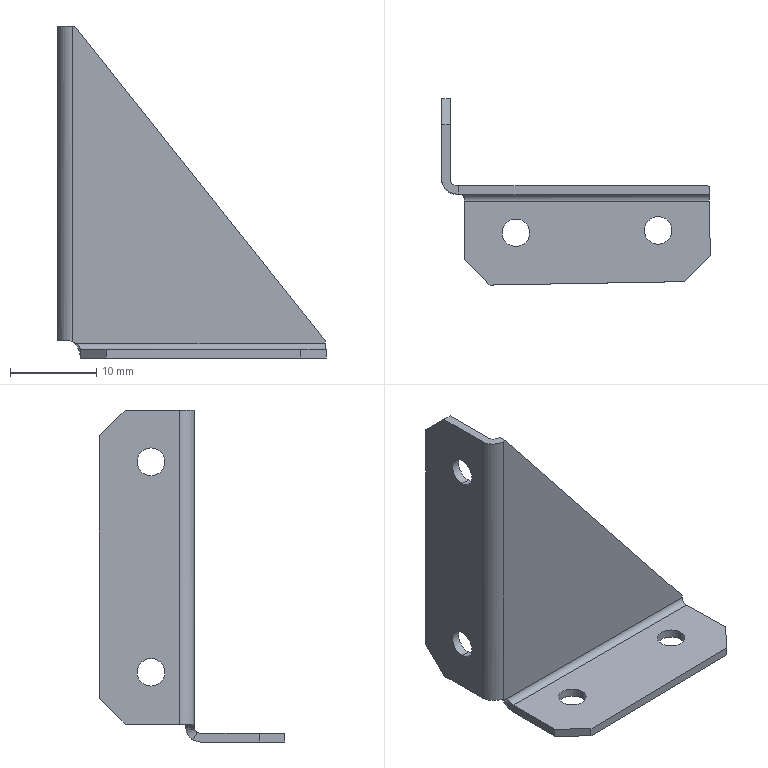Part | SolidWorks | features BaseBody 1 | 1 solid | 34 faces | box 31.131 x 21.506 x 38.476 mm | volume 1233 mm3 | plane 18 | cylinder 13 | spline 3 | commonest cylinder face diameters 3.2 x9 1.473 x2 3.473 x2
STEP:
#1=CARTESIAN_POINT('',(6.,-5.422,0.5237));
#2=VERTEX_POINT('',#1);
#3=CARTESIAN_POINT('',(9.2,-5.422,0.5237));
#4=VERTEX_POINT('',#3);
#5=CARTESIAN_POINT('',(7.6,-5.422,0.5237));
#6=DIRECTION('',(0.,0.,1.));
#7=DIRECTION('',(-1.,0.,0.));
#8=AXIS2_PLACEMENT_3D('',#5,#6,#7);
#9=CIRCLE('',#8,1.6);
#10=EDGE_CURVE('',#2,#4,#9,.T.);
#11=ORIENTED_EDGE('',*,*,#10,.T.);
#12=CARTESIAN_POINT('',(9.2,-5.422,-0.4763));
#13=VERTEX_POINT('',#12);
#14=CARTESIAN_POINT('',(9.2,-5.422,0.5237));
#15=DIRECTION('',(0.,0.,-1.));
#16=VECTOR('',#15,1000.);
#17=LINE('',#14,#16);
#18=EDGE_CURVE('',#4,#13,#17,.T.);
#19=ORIENTED_EDGE('',*,*,#18,.T.);
#20=CARTESIAN_POINT('',(6.,-5.422,-0.4763));
#21=VERTEX_POINT('',#20);
#22=CARTESIAN_POINT('',(7.6,-5.422,-0.4763));
#23=DIRECTION('',(0.,0.,-1.));
#24=DIRECTION('',(-1.,0.,0.));
#25=AXIS2_PLACEMENT_3D('',#22,#23,#24);
#26=CIRCLE('',#25,1.6);
#27=EDGE_CURVE('',#13,#21,#26,.T.);
#28=ORIENTED_EDGE('',*,*,#27,.T.);
#29=CARTESIAN_POINT('',(6.,-5.422,0.5237));
#30=DIRECTION('',(0.,0.,-1.));
#31=VECTOR('',#30,1000.);
#32=LINE('',#29,#31);
#33=EDGE_CURVE('',#2,#21,#32,.T.);
#34=ORIENTED_EDGE('',*,*,#33,.F.);
#35=EDGE_LOOP('',(#11,#19,#28,#34));
#36=FACE_OUTER_BOUND('',#35,.T.);
#37=CARTESIAN_POINT('',(7.6,-5.422,0.5237));
#38=DIRECTION('',(0.,0.,-1.));
#39=DIRECTION('',(-1.,0.,0.));
#40=AXIS2_PLACEMENT_3D('',#37,#38,#39);
#41=CYLINDRICAL_SURFACE('',#40,1.6);
#42=ADVANCED_FACE('',(#36),#41,.F.);
#43=CARTESIAN_POINT('',(22.479,-5.135,0.5237));
#44=VERTEX_POINT('',#43);
#45=CARTESIAN_POINT('',(25.679,-5.135,0.5237));
#46=VERTEX_POINT('',#45);
#47=CARTESIAN_POINT('',(24.079,-5.135,0.5237));
#48=DIRECTION('',(0.,0.,1.));
#49=DIRECTION('',(-1.,0.,0.));
#50=AXIS2_PLACEMENT_3D('',#47,#48,#49);
#51=CIRCLE('',#50,1.6);
#52=EDGE_CURVE('',#44,#46,#51,.T.);
#53=ORIENTED_EDGE('',*,*,#52,.T.);
#54=CARTESIAN_POINT('',(25.679,-5.135,-0.4763));
#55=VERTEX_POINT('',#54);
#56=CARTESIAN_POINT('',(25.679,-5.135,0.5237));
#57=DIRECTION('',(0.,0.,-1.));
#58=VECTOR('',#57,1000.);
#59=LINE('',#56,#58);
#60=EDGE_CURVE('',#46,#55,#59,.T.);
#61=ORIENTED_EDGE('',*,*,#60,.T.);
#62=CARTESIAN_POINT('',(22.479,-5.135,-0.4763));
#63=VERTEX_POINT('',#62);
#64=CARTESIAN_POINT('',(24.079,-5.135,-0.4763));
#65=DIRECTION('',(0.,0.,1.));
#66=DIRECTION('',(-1.,0.,0.));
#67=AXIS2_PLACEMENT_3D('',#64,#65,#66);
#68=CIRCLE('',#67,1.6);
#69=EDGE_CURVE('',#63,#55,#68,.T.);
#70=ORIENTED_EDGE('',*,*,#69,.F.);
#71=CARTESIAN_POINT('',(22.479,-5.135,0.5237));
#72=DIRECTION('',(0.,0.,-1.));
#73=VECTOR('',#72,1000.);
#74=LINE('',#71,#73);
#75=EDGE_CURVE('',#44,#63,#74,.T.);
#76=ORIENTED_EDGE('',*,*,#75,.F.);
#77=EDGE_LOOP('',(#53,#61,#70,#76));
#78=FACE_OUTER_BOUND('',#77,.T.);
#79=CARTESIAN_POINT('',(24.079,-5.135,0.5237));
#80=DIRECTION('',(0.,0.,-1.));
#81=DIRECTION('',(-1.,0.,0.));
#82=AXIS2_PLACEMENT_3D('',#79,#80,#81);
#83=CYLINDRICAL_SURFACE('',#82,1.6);
#84=ADVANCED_FACE('',(#78),#83,.F.);
#85=CARTESIAN_POINT('',(-1.,4.031,6.));
#86=VERTEX_POINT('',#85);
#87=CARTESIAN_POINT('',(-1.,4.031,9.2));
#88=VERTEX_POINT('',#87);
#89=CARTESIAN_POINT('',(-1.,4.031,7.6));
#90=DIRECTION('',(-1.,0.,0.));
#91=DIRECTION('',(0.,0.,-1.));
#92=AXIS2_PLACEMENT_3D('',#89,#90,#91);
#93=CIRCLE('',#92,1.6);
#94=EDGE_CURVE('',#86,#88,#93,.T.);
#95=ORIENTED_EDGE('',*,*,#94,.T.);
#96=CARTESIAN_POINT('',(0.,4.031,9.2));
#97=VERTEX_POINT('',#96);
#98=CARTESIAN_POINT('',(-1.,4.031,9.2));
#99=DIRECTION('',(1.,0.,0.));
#100=VECTOR('',#99,1000.);
#101=LINE('',#98,#100);
#102=EDGE_CURVE('',#88,#97,#101,.T.);
#103=ORIENTED_EDGE('',*,*,#102,.T.);
#104=CARTESIAN_POINT('',(0.,4.031,6.));
#105=VERTEX_POINT('',#104);
#106=CARTESIAN_POINT('',(0.,4.031,7.6));
#107=DIRECTION('',(-1.,0.,0.));
#108=DIRECTION('',(0.,0.,-1.));
#109=AXIS2_PLACEMENT_3D('',#106,#107,#108);
#110=CIRCLE('',#109,1.6);
#111=EDGE_CURVE('',#105,#97,#110,.T.);
#112=ORIENTED_EDGE('',*,*,#111,.F.);
#113=CARTESIAN_POINT('',(-1.,4.031,6.));
#114=DIRECTION('',(1.,0.,0.));
#115=VECTOR('',#114,1000.);
#116=LINE('',#113,#115);
#117=EDGE_CURVE('',#86,#105,#116,.T.);
#118=ORIENTED_EDGE('',*,*,#117,.F.);
#119=EDGE_LOOP('',(#95,#103,#112,#118));
#120=FACE_OUTER_BOUND('',#119,.T.);
#121=CARTESIAN_POINT('',(-1.,4.031,7.6));
#122=DIRECTION('',(1.,0.,0.));
#123=DIRECTION('',(0.,0.,-1.));
#124=AXIS2_PLACEMENT_3D('',#121,#122,#123);
#125=CYLINDRICAL_SURFACE('',#124,1.6);
#126=ADVANCED_FACE('',(#120),#125,.F.);
#127=CARTESIAN_POINT('',(-1.,4.031,30.4));
#128=VERTEX_POINT('',#127);
#129=CARTESIAN_POINT('',(-1.,4.031,33.6));
#130=VERTEX_POINT('',#129);
#131=CARTESIAN_POINT('',(-1.,4.031,32.));
#132=DIRECTION('',(-1.,0.,0.));
#133=DIRECTION('',(0.,0.,-1.));
#134=AXIS2_PLACEMENT_3D('',#131,#132,#133);
#135=CIRCLE('',#134,1.6);
#136=EDGE_CURVE('',#128,#130,#135,.T.);
#137=ORIENTED_EDGE('',*,*,#136,.T.);
#138=CARTESIAN_POINT('',(0.,4.031,33.6));
#139=VERTEX_POINT('',#138);
#140=CARTESIAN_POINT('',(-1.,4.031,33.6));
#141=DIRECTION('',(1.,0.,0.));
#142=VECTOR('',#141,1000.);
#143=LINE('',#140,#142);
#144=EDGE_CURVE('',#130,#139,#143,.T.);
#145=ORIENTED_EDGE('',*,*,#144,.T.);
#146=CARTESIAN_POINT('',(0.,4.031,30.4));
#147=VERTEX_POINT('',#146);
#148=CARTESIAN_POINT('',(0.,4.031,32.));
#149=DIRECTION('',(-1.,0.,0.));
#150=DIRECTION('',(0.,0.,-1.));
#151=AXIS2_PLACEMENT_3D('',#148,#149,#150);
#152=CIRCLE('',#151,1.6);
#153=EDGE_CURVE('',#147,#139,#152,.T.);
#154=ORIENTED_EDGE('',*,*,#153,.F.);
#155=CARTESIAN_POINT('',(-1.,4.031,30.4));
#156=DIRECTION('',(1.,0.,0.));
#157=VECTOR('',#156,1000.);
#158=LINE('',#155,#157);
#159=EDGE_CURVE('',#128,#147,#158,.T.);
#160=ORIENTED_EDGE('',*,*,#159,.F.);
#161=EDGE_LOOP('',(#137,#145,#154,#160));
#162=FACE_OUTER_BOUND('',#161,.T.);
#163=CARTESIAN_POINT('',(-1.,4.031,32.));
#164=DIRECTION('',(1.,0.,0.));
#165=DIRECTION('',(0.,0.,-1.));
#166=AXIS2_PLACEMENT_3D('',#163,#164,#165);
#167=CYLINDRICAL_SURFACE('',#166,1.6);
#168=ADVANCED_FACE('',(#162),#167,.F.);
#169=ORIENTED_EDGE('',*,*,#18,.F.);
#170=CARTESIAN_POINT('',(7.6,-5.422,0.5237));
#171=DIRECTION('',(0.,0.,1.));
#172=DIRECTION('',(-1.,0.,0.));
#173=AXIS2_PLACEMENT_3D('',#170,#171,#172);
#174=CIRCLE('',#173,1.6);
#175=EDGE_CURVE('',#4,#2,#174,.T.);
#176=ORIENTED_EDGE('',*,*,#175,.T.);
#177=ORIENTED_EDGE('',*,*,#33,.T.);
#178=CARTESIAN_POINT('',(7.6,-5.422,-0.4763));
#179=DIRECTION('',(0.,0.,-1.));
#180=DIRECTION('',(-1.,0.,0.));
#181=AXIS2_PLACEMENT_3D('',#178,#179,#180);
#182=CIRCLE('',#181,1.6);
#183=EDGE_CURVE('',#21,#13,#182,.T.);
#184=ORIENTED_EDGE('',*,*,#183,.T.);
#185=EDGE_LOOP('',(#169,#176,#177,#184));
#186=FACE_OUTER_BOUND('',#185,.T.);
#187=CARTESIAN_POINT('',(7.6,-5.422,0.5237));
#188=DIRECTION('',(0.,0.,-1.));
#189=DIRECTION('',(-1.,0.,0.));
#190=AXIS2_PLACEMENT_3D('',#187,#188,#189);
#191=CYLINDRICAL_SURFACE('',#190,1.6);
#192=ADVANCED_FACE('',(#186),#191,.F.);
#193=ORIENTED_EDGE('',*,*,#183,.F.);
#194=ORIENTED_EDGE('',*,*,#27,.F.);
#195=EDGE_LOOP('',(#193,#194));
#196=FACE_BOUND('',#195,.T.);
#197=ORIENTED_EDGE('',*,*,#69,.T.);
#198=CARTESIAN_POINT('',(24.079,-5.135,-0.4763));
#199=DIRECTION('',(0.,0.,1.));
#200=DIRECTION('',(-1.,0.,0.));
#201=AXIS2_PLACEMENT_3D('',#198,#199,#200);
#202=CIRCLE('',#201,1.6);
#203=EDGE_CURVE('',#55,#63,#202,.T.);
#204=ORIENTED_EDGE('',*,*,#203,.T.);
#205=EDGE_LOOP('',(#197,#204));
#206=FACE_BOUND('',#205,.T.);
#207=CARTESIAN_POINT('',(4.6,-11.476,-0.4763));
#208=VERTEX_POINT('',#207);
#209=CARTESIAN_POINT('',(1.6,-8.528,-0.4763));
#210=VERTEX_POINT('',#209);
#211=CARTESIAN_POINT('',(4.6,-11.476,-0.4763));
#212=DIRECTION('',(-0.7133,0.7009,0.));
#213=VECTOR('',#212,1000.);
#214=LINE('',#211,#213);
#215=EDGE_CURVE('',#208,#210,#214,.T.);
#216=ORIENTED_EDGE('',*,*,#215,.T.);
#217=CARTESIAN_POINT('',(1.6,-1.737,-0.4763));
#218=VERTEX_POINT('',#217);
#219=CARTESIAN_POINT('',(1.6,-6.635,-0.4763));
#220=DIRECTION('',(0.,1.,0.));
#221=VECTOR('',#220,1000.);
#222=LINE('',#219,#221);
#223=EDGE_CURVE('',#210,#218,#222,.T.);
#224=ORIENTED_EDGE('',*,*,#223,.T.);
#225=CARTESIAN_POINT('',(30.021,-1.737,-0.4763));
#226=VERTEX_POINT('',#225);
#227=CARTESIAN_POINT('',(15.951,-1.737,-0.4763));
#228=DIRECTION('',(1.,0.,0.));
#229=VECTOR('',#228,1000.);
#230=LINE('',#227,#229);
#231=EDGE_CURVE('',#218,#226,#230,.T.);
#232=ORIENTED_EDGE('',*,*,#231,.T.);
#233=CARTESIAN_POINT('',(30.131,-8.03,-0.4763));
#234=VERTEX_POINT('',#233);
#235=CARTESIAN_POINT('',(30.021,-1.737,-0.4763));
#236=DIRECTION('',(0.01745,-0.9998,0.));
#237=VECTOR('',#236,1000.);
#238=LINE('',#235,#237);
#239=EDGE_CURVE('',#226,#234,#238,.T.);
#240=ORIENTED_EDGE('',*,*,#239,.T.);
#241=CARTESIAN_POINT('',(27.184,-11.082,-0.4763));
#242=VERTEX_POINT('',#241);
#243=CARTESIAN_POINT('',(30.131,-8.03,-0.4763));
#244=DIRECTION('',(-0.6947,-0.7193,0.));
#245=VECTOR('',#244,1000.);
#246=LINE('',#243,#245);
#247=EDGE_CURVE('',#234,#242,#246,.T.);
#248=ORIENTED_EDGE('',*,*,#247,.T.);
#249=CARTESIAN_POINT('',(27.184,-11.082,-0.4763));
#250=DIRECTION('',(-0.9998,-0.01745,0.));
#251=VECTOR('',#250,1000.);
#252=LINE('',#249,#251);
#253=EDGE_CURVE('',#242,#208,#252,.T.);
#254=ORIENTED_EDGE('',*,*,#253,.T.);
#255=EDGE_LOOP('',(#216,#224,#232,#240,#248,#254));
#256=FACE_OUTER_BOUND('',#255,.T.);
#257=CARTESIAN_POINT('',(30.302,-1.737,-0.4763));
#258=DIRECTION('',(0.,0.,-1.));
#259=DIRECTION('',(0.,-1.,0.));
#260=AXIS2_PLACEMENT_3D('',#257,#258,#259);
#261=PLANE('',#260);
#262=ADVANCED_FACE('',(#196,#206,#256),#261,.T.);
#263=ORIENTED_EDGE('',*,*,#52,.F.);
#264=CARTESIAN_POINT('',(24.079,-5.135,0.5237));
#265=DIRECTION('',(0.,0.,1.));
#266=DIRECTION('',(-1.,0.,0.));
#267=AXIS2_PLACEMENT_3D('',#264,#265,#266);
#268=CIRCLE('',#267,1.6);
#269=EDGE_CURVE('',#46,#44,#268,.T.);
#270=ORIENTED_EDGE('',*,*,#269,.F.);
#271=EDGE_LOOP('',(#263,#270));
#272=FACE_BOUND('',#271,.T.);
#273=ORIENTED_EDGE('',*,*,#10,.F.);
#274=ORIENTED_EDGE('',*,*,#175,.F.);
#275=EDGE_LOOP('',(#273,#274));
#276=FACE_BOUND('',#275,.T.);
#277=CARTESIAN_POINT('',(4.6,-11.476,0.5237));
#278=VERTEX_POINT('',#277);
#279=CARTESIAN_POINT('',(1.6,-8.528,0.5237));
#280=VERTEX_POINT('',#279);
#281=CARTESIAN_POINT('',(1.6,-8.528,0.5237));
#282=DIRECTION('',(-0.7133,0.7009,0.));
#283=VECTOR('',#282,1000.);
#284=LINE('',#281,#283);
#285=EDGE_CURVE('',#278,#280,#284,.T.);
#286=ORIENTED_EDGE('',*,*,#285,.F.);
#287=CARTESIAN_POINT('',(27.184,-11.082,0.5237));
#288=VERTEX_POINT('',#287);
#289=CARTESIAN_POINT('',(4.6,-11.476,0.5237));
#290=DIRECTION('',(-0.9998,-0.01745,0.));
#291=VECTOR('',#290,1000.);
#292=LINE('',#289,#291);
#293=EDGE_CURVE('',#288,#278,#292,.T.);
#294=ORIENTED_EDGE('',*,*,#293,.F.);
#295=CARTESIAN_POINT('',(30.131,-8.03,0.5237));
#296=VERTEX_POINT('',#295);
#297=CARTESIAN_POINT('',(27.184,-11.082,0.5237));
#298=DIRECTION('',(-0.6947,-0.7193,0.));
#299=VECTOR('',#298,1000.);
#300=LINE('',#297,#299);
#301=EDGE_CURVE('',#296,#288,#300,.T.);
#302=ORIENTED_EDGE('',*,*,#301,.F.);
#303=CARTESIAN_POINT('',(30.021,-1.737,0.5237));
#304=VERTEX_POINT('',#303);
#305=CARTESIAN_POINT('',(30.131,-8.03,0.5237));
#306=DIRECTION('',(0.01745,-0.9998,0.));
#307=VECTOR('',#306,1000.);
#308=LINE('',#305,#307);
#309=EDGE_CURVE('',#304,#296,#308,.T.);
#310=ORIENTED_EDGE('',*,*,#309,.F.);
#311=CARTESIAN_POINT('',(1.6,-1.737,0.5237));
#312=VERTEX_POINT('',#311);
#313=CARTESIAN_POINT('',(15.951,-1.737,0.5237));
#314=DIRECTION('',(1.,0.,0.));
#315=VECTOR('',#314,1000.);
#316=LINE('',#313,#315);
#317=EDGE_CURVE('',#312,#304,#316,.T.);
#318=ORIENTED_EDGE('',*,*,#317,.F.);
#319=CARTESIAN_POINT('',(1.6,-6.635,0.5237));
#320=DIRECTION('',(0.,1.,0.));
#321=VECTOR('',#320,1000.);
#322=LINE('',#319,#321);
#323=EDGE_CURVE('',#280,#312,#322,.T.);
#324=ORIENTED_EDGE('',*,*,#323,.F.);
#325=EDGE_LOOP('',(#286,#294,#302,#310,#318,#324));
#326=FACE_OUTER_BOUND('',#325,.T.);
#327=CARTESIAN_POINT('',(30.302,-1.737,0.5237));
#328=DIRECTION('',(0.,0.,-1.));
#329=DIRECTION('',(0.,-1.,0.));
#330=AXIS2_PLACEMENT_3D('',#327,#328,#329);
#331=PLANE('',#330);
#332=ADVANCED_FACE('',(#272,#276,#326),#331,.F.);
#333=ORIENTED_EDGE('',*,*,#60,.F.);
#334=ORIENTED_EDGE('',*,*,#269,.T.);
#335=ORIENTED_EDGE('',*,*,#75,.T.);
#336=ORIENTED_EDGE('',*,*,#203,.F.);
#337=EDGE_LOOP('',(#333,#334,#335,#336));
#338=FACE_OUTER_BOUND('',#337,.T.);
#339=CARTESIAN_POINT('',(24.079,-5.135,0.5237));
#340=DIRECTION('',(0.,0.,-1.));
#341=DIRECTION('',(-1.,0.,0.));
#342=AXIS2_PLACEMENT_3D('',#339,#340,#341);
#343=CYLINDRICAL_SURFACE('',#342,1.6);
#344=ADVANCED_FACE('',(#338),#343,.F.);
#345=CARTESIAN_POINT('',(1.6,-8.528,0.02365));
#346=DIRECTION('',(0.,0.,1.));
#347=VECTOR('',#346,1000.);
#348=LINE('',#345,#347);
#349=EDGE_CURVE('',#210,#280,#348,.T.);
#350=ORIENTED_EDGE('',*,*,#349,.T.);
#351=ORIENTED_EDGE('',*,*,#323,.T.);
#352=CARTESIAN_POINT('',(1.6,-1.351,0.6329));
#353=VERTEX_POINT('',#352);
#354=CARTESIAN_POINT('',(1.6,-1.737,1.26));
#355=DIRECTION('',(-1.,0.,0.));
#356=DIRECTION('',(0.,-1.,0.));
#357=AXIS2_PLACEMENT_3D('',#354,#355,#356);
#358=CIRCLE('',#357,0.7366);
#359=EDGE_CURVE('',#353,#312,#358,.T.);
#360=ORIENTED_EDGE('',*,*,#359,.F.);
#361=CARTESIAN_POINT('',(1.6,-0.8264,-0.2187));
#362=VERTEX_POINT('',#361);
#363=CARTESIAN_POINT('',(1.6,-1.351,0.6329));
#364=DIRECTION('',(0.,-0.5241,0.8517));
#365=VECTOR('',#364,1000.);
#366=LINE('',#363,#365);
#367=EDGE_CURVE('',#362,#353,#366,.T.);
#368=ORIENTED_EDGE('',*,*,#367,.F.);
#369=CARTESIAN_POINT('',(1.6,-1.737,1.26));
#370=DIRECTION('',(-1.,0.,0.));
#371=DIRECTION('',(0.,-1.,0.));
#372=AXIS2_PLACEMENT_3D('',#369,#370,#371);
#373=CIRCLE('',#372,1.737);
#374=EDGE_CURVE('',#362,#218,#373,.T.);
#375=ORIENTED_EDGE('',*,*,#374,.T.);
#376=ORIENTED_EDGE('',*,*,#223,.F.);
#377=EDGE_LOOP('',(#350,#351,#360,#368,#375,#376));
#378=FACE_OUTER_BOUND('',#377,.T.);
#379=CARTESIAN_POINT('',(1.6,-1.737,-0.4763));
#380=DIRECTION('',(-1.,0.,0.));
#381=DIRECTION('',(0.,-1.,0.));
#382=AXIS2_PLACEMENT_3D('',#379,#380,#381);
#383=PLANE('',#382);
#384=ADVANCED_FACE('',(#378),#383,.T.);
#385=ORIENTED_EDGE('',*,*,#285,.T.);
#386=ORIENTED_EDGE('',*,*,#349,.F.);
#387=ORIENTED_EDGE('',*,*,#215,.F.);
#388=CARTESIAN_POINT('',(4.6,-11.476,0.02365));
#389=DIRECTION('',(0.,0.,1.));
#390=VECTOR('',#389,1000.);
#391=LINE('',#388,#390);
#392=EDGE_CURVE('',#208,#278,#391,.T.);
#393=ORIENTED_EDGE('',*,*,#392,.T.);
#394=EDGE_LOOP('',(#385,#386,#387,#393));
#395=FACE_OUTER_BOUND('',#394,.T.);
#396=CARTESIAN_POINT('',(1.6,-8.528,-0.4763));
#397=DIRECTION('',(-0.7009,-0.7133,0.));
#398=DIRECTION('',(0.7133,-0.7009,0.));
#399=AXIS2_PLACEMENT_3D('',#396,#397,#398);
#400=PLANE('',#399);
#401=ADVANCED_FACE('',(#395),#400,.T.);
#402=ORIENTED_EDGE('',*,*,#293,.T.);
#403=ORIENTED_EDGE('',*,*,#392,.F.);
#404=ORIENTED_EDGE('',*,*,#253,.F.);
#405=CARTESIAN_POINT('',(27.184,-11.082,0.02365));
#406=DIRECTION('',(0.,0.,1.));
#407=VECTOR('',#406,1000.);
#408=LINE('',#405,#407);
#409=EDGE_CURVE('',#242,#288,#408,.T.);
#410=ORIENTED_EDGE('',*,*,#409,.T.);
#411=EDGE_LOOP('',(#402,#403,#404,#410));
#412=FACE_OUTER_BOUND('',#411,.T.);
#413=CARTESIAN_POINT('',(4.6,-11.476,-0.4763));
#414=DIRECTION('',(0.01745,-0.9998,0.));
#415=DIRECTION('',(0.9998,0.01745,0.));
#416=AXIS2_PLACEMENT_3D('',#413,#414,#415);
#417=PLANE('',#416);
#418=ADVANCED_FACE('',(#412),#417,.T.);
#419=ORIENTED_EDGE('',*,*,#301,.T.);
#420=ORIENTED_EDGE('',*,*,#409,.F.);
#421=ORIENTED_EDGE('',*,*,#247,.F.);
#422=CARTESIAN_POINT('',(30.131,-8.03,0.02365));
#423=DIRECTION('',(0.,0.,1.));
#424=VECTOR('',#423,1000.);
#425=LINE('',#422,#424);
#426=EDGE_CURVE('',#234,#296,#425,.T.);
#427=ORIENTED_EDGE('',*,*,#426,.T.);
#428=EDGE_LOOP('',(#419,#420,#421,#427));
#429=FACE_OUTER_BOUND('',#428,.T.);
#430=CARTESIAN_POINT('',(27.184,-11.082,-0.4763));
#431=DIRECTION('',(0.7193,-0.6947,0.));
#432=DIRECTION('',(0.6947,0.7193,0.));
#433=AXIS2_PLACEMENT_3D('',#430,#431,#432);
#434=PLANE('',#433);
#435=ADVANCED_FACE('',(#429),#434,.T.);
#436=ORIENTED_EDGE('',*,*,#426,.F.);
#437=ORIENTED_EDGE('',*,*,#239,.F.);
#438=CARTESIAN_POINT('',(30.021,-1.737,0.02365));
#439=DIRECTION('',(0.,0.,1.));
#440=VECTOR('',#439,1000.);
#441=LINE('',#438,#440);
#442=EDGE_CURVE('',#226,#304,#441,.T.);
#443=ORIENTED_EDGE('',*,*,#442,.T.);
#444=ORIENTED_EDGE('',*,*,#309,.T.);
#445=EDGE_LOOP('',(#436,#437,#443,#444));
#446=FACE_OUTER_BOUND('',#445,.T.);
#447=CARTESIAN_POINT('',(30.131,-8.03,-0.4763));
#448=DIRECTION('',(0.9998,0.01745,0.));
#449=DIRECTION('',(-0.01745,0.9998,0.));
#450=AXIS2_PLACEMENT_3D('',#447,#448,#449);
#451=PLANE('',#450);
#452=ADVANCED_FACE('',(#446),#451,.T.);
#453=CARTESIAN_POINT('',(30.,-0.2991,0.2859));
#454=VERTEX_POINT('',#453);
#455=CARTESIAN_POINT('',(30.021,-1.737,-0.4763));
#456=CARTESIAN_POINT('',(30.018,-1.454,-0.4763));
#457=CARTESIAN_POINT('',(30.014,-1.172,-0.4062));
#458=CARTESIAN_POINT('',(30.007,-0.6737,-0.1418));
#459=CARTESIAN_POINT('',(30.004,-0.4574,0.05229));
#460=CARTESIAN_POINT('',(30.,-0.2991,0.2859));
#461=B_SPLINE_CURVE_WITH_KNOTS('',3,(#455,#456,#457,#458,#459,#460),.UNSPECIFIED.,.F.,.F.,(4,2,4),(0.,0.5,1.),.UNSPECIFIED.);
#462=EDGE_CURVE('',#226,#454,#461,.T.);
#463=ORIENTED_EDGE('',*,*,#462,.F.);
#464=ORIENTED_EDGE('',*,*,#231,.F.);
#465=ORIENTED_EDGE('',*,*,#374,.F.);
#466=CARTESIAN_POINT('',(0.9858,0.,1.26));
#467=VERTEX_POINT('',#466);
#468=CARTESIAN_POINT('',(0.9858,0.,1.26));
#469=CARTESIAN_POINT('',(1.078,0.,1.13));
#470=CARTESIAN_POINT('',(1.165,-0.01435,0.9991));
#471=CARTESIAN_POINT('',(1.323,-0.07617,0.7336));
#472=CARTESIAN_POINT('',(1.396,-0.1248,0.5968));
#473=CARTESIAN_POINT('',(1.475,-0.2271,0.3984));
#474=CARTESIAN_POINT('',(1.495,-0.2663,0.3328));
#475=CARTESIAN_POINT('',(1.524,-0.3562,0.2037));
#476=CARTESIAN_POINT('',(1.536,-0.406,0.1415));
#477=CARTESIAN_POINT('',(1.567,-0.5665,-0.03262));
#478=CARTESIAN_POINT('',(1.584,-0.6903,-0.1349));
#479=CARTESIAN_POINT('',(1.6,-0.8264,-0.2187));
#480=B_SPLINE_CURVE_WITH_KNOTS('',3,(#468,#469,#470,#471,#472,#473,#474,#475,#476,#477,#478,#479),.UNSPECIFIED.,.F.,.F.,(4,2,2,2,2,4),(0.,0.0004721,0.0009441,0.00118,0.001416,0.001888),.UNSPECIFIED.);
#481=EDGE_CURVE('',#467,#362,#480,.T.);
#482=ORIENTED_EDGE('',*,*,#481,.F.);
#483=CARTESIAN_POINT('',(30.,0.,1.26));
#484=VERTEX_POINT('',#483);
#485=CARTESIAN_POINT('',(15.503,0.,1.26));
#486=DIRECTION('',(-1.,0.,0.));
#487=VECTOR('',#486,1000.);
#488=LINE('',#485,#487);
#489=EDGE_CURVE('',#484,#467,#488,.T.);
#490=ORIENTED_EDGE('',*,*,#489,.F.);
#491=CARTESIAN_POINT('',(30.,-1.737,1.26));
#492=DIRECTION('',(1.,0.,0.));
#493=DIRECTION('',(0.,-1.,0.));
#494=AXIS2_PLACEMENT_3D('',#491,#492,#493);
#495=CIRCLE('',#494,1.737);
#496=EDGE_CURVE('',#454,#484,#495,.T.);
#497=ORIENTED_EDGE('',*,*,#496,.F.);
#498=EDGE_LOOP('',(#463,#464,#465,#482,#490,#497));
#499=FACE_OUTER_BOUND('',#498,.T.);
#500=CARTESIAN_POINT('',(30.195,-1.737,1.26));
#501=DIRECTION('',(-1.,0.,0.));
#502=DIRECTION('',(0.,-1.,0.));
#503=AXIS2_PLACEMENT_3D('',#500,#501,#502);
#504=CYLINDRICAL_SURFACE('',#503,1.737);
#505=ADVANCED_FACE('',(#499),#504,.T.);
#506=ORIENTED_EDGE('',*,*,#317,.T.);
#507=CARTESIAN_POINT('',(30.,-1.127,0.847));
#508=VERTEX_POINT('',#507);
#509=CARTESIAN_POINT('',(30.021,-1.737,0.5237));
#510=CARTESIAN_POINT('',(30.018,-1.617,0.5237));
#511=CARTESIAN_POINT('',(30.014,-1.497,0.5534));
#512=CARTESIAN_POINT('',(30.007,-1.286,0.6656));
#513=CARTESIAN_POINT('',(30.004,-1.194,0.7479));
#514=CARTESIAN_POINT('',(30.,-1.127,0.847));
#515=B_SPLINE_CURVE_WITH_KNOTS('',3,(#509,#510,#511,#512,#513,#514),.UNSPECIFIED.,.F.,.F.,(4,2,4),(0.,0.5,1.),.UNSPECIFIED.);
#516=EDGE_CURVE('',#304,#508,#515,.T.);
#517=ORIENTED_EDGE('',*,*,#516,.T.);
#518=CARTESIAN_POINT('',(30.,-1.,1.26));
#519=VERTEX_POINT('',#518);
#520=CARTESIAN_POINT('',(30.,-1.737,1.26));
#521=DIRECTION('',(1.,0.,0.));
#522=DIRECTION('',(0.,-1.,0.));
#523=AXIS2_PLACEMENT_3D('',#520,#521,#522);
#524=CIRCLE('',#523,0.7366);
#525=EDGE_CURVE('',#508,#519,#524,.T.);
#526=ORIENTED_EDGE('',*,*,#525,.T.);
#527=CARTESIAN_POINT('',(0.9858,-1.,1.26));
#528=VERTEX_POINT('',#527);
#529=CARTESIAN_POINT('',(15.503,-1.,1.26));
#530=DIRECTION('',(-1.,0.,0.));
#531=VECTOR('',#530,1000.);
#532=LINE('',#529,#531);
#533=EDGE_CURVE('',#519,#528,#532,.T.);
#534=ORIENTED_EDGE('',*,*,#533,.T.);
#535=CARTESIAN_POINT('',(0.9858,-1.,1.26));
#536=CARTESIAN_POINT('',(1.059,-1.,1.217));
#537=CARTESIAN_POINT('',(1.13,-1.004,1.172));
#538=CARTESIAN_POINT('',(1.269,-1.022,1.076));
#539=CARTESIAN_POINT('',(1.337,-1.036,1.027));
#540=CARTESIAN_POINT('',(1.427,-1.07,0.9455));
#541=CARTESIAN_POINT('',(1.456,-1.084,0.917));
#542=CARTESIAN_POINT('',(1.503,-1.12,0.8557));
#543=CARTESIAN_POINT('',(1.519,-1.142,0.8234));
#544=CARTESIAN_POINT('',(1.56,-1.218,0.7311));
#545=CARTESIAN_POINT('',(1.58,-1.28,0.6762));
#546=CARTESIAN_POINT('',(1.6,-1.351,0.6329));
#547=B_SPLINE_CURVE_WITH_KNOTS('',3,(#535,#536,#537,#538,#539,#540,#541,#542,#543,#544,#545,#546),.UNSPECIFIED.,.F.,.F.,(4,2,2,2,2,4),(0.,0.000254,0.000508,0.000635,0.000762,0.001016),.UNSPECIFIED.);
#548=EDGE_CURVE('',#528,#353,#547,.T.);
#549=ORIENTED_EDGE('',*,*,#548,.T.);
#550=ORIENTED_EDGE('',*,*,#359,.T.);
#551=EDGE_LOOP('',(#506,#517,#526,#534,#549,#550));
#552=FACE_OUTER_BOUND('',#551,.T.);
#553=CARTESIAN_POINT('',(30.195,-1.737,1.26));
#554=DIRECTION('',(-1.,0.,0.));
#555=DIRECTION('',(0.,-1.,0.));
#556=AXIS2_PLACEMENT_3D('',#553,#554,#555);
#557=CYLINDRICAL_SURFACE('',#556,0.7366);
#558=ADVANCED_FACE('',(#552),#557,.F.);
#559=ORIENTED_EDGE('',*,*,#516,.F.);
#560=ORIENTED_EDGE('',*,*,#442,.F.);
#561=ORIENTED_EDGE('',*,*,#462,.T.);
#562=CARTESIAN_POINT('',(30.,-0.713,0.5664));
#563=DIRECTION('',(0.,-0.8278,0.5611));
#564=VECTOR('',#563,1000.);
#565=LINE('',#562,#564);
#566=EDGE_CURVE('',#454,#508,#565,.T.);
#567=ORIENTED_EDGE('',*,*,#566,.T.);
#568=EDGE_LOOP('',(#559,#560,#561,#567));
#569=FACE_OUTER_BOUND('',#568,.T.);
#570=CARTESIAN_POINT('',(30.,-0.2908,0.2803));
#571=CARTESIAN_POINT('',(30.004,-0.4501,0.04523));
#572=CARTESIAN_POINT('',(30.007,-0.6676,-0.1498));
#573=CARTESIAN_POINT('',(30.014,-1.169,-0.4158));
#574=CARTESIAN_POINT('',(30.018,-1.453,-0.4863));
#575=CARTESIAN_POINT('',(30.021,-1.737,-0.4863));
#576=CARTESIAN_POINT('',(30.,-0.2991,0.2859));
#577=CARTESIAN_POINT('',(30.004,-0.4575,0.05219));
#578=CARTESIAN_POINT('',(30.007,-0.6737,-0.1418));
#579=CARTESIAN_POINT('',(30.014,-1.172,-0.4062));
#580=CARTESIAN_POINT('',(30.018,-1.454,-0.4763));
#581=CARTESIAN_POINT('',(30.021,-1.737,-0.4763));
#582=CARTESIAN_POINT('',(30.,-1.127,0.847));
#583=CARTESIAN_POINT('',(30.004,-1.194,0.7478));
#584=CARTESIAN_POINT('',(30.007,-1.286,0.6656));
#585=CARTESIAN_POINT('',(30.014,-1.497,0.5534));
#586=CARTESIAN_POINT('',(30.018,-1.617,0.5237));
#587=CARTESIAN_POINT('',(30.021,-1.737,0.5237));
#588=CARTESIAN_POINT('',(30.,-1.135,0.8526));
#589=CARTESIAN_POINT('',(30.004,-1.201,0.7549));
#590=CARTESIAN_POINT('',(30.007,-1.292,0.6737));
#591=CARTESIAN_POINT('',(30.014,-1.501,0.5631));
#592=CARTESIAN_POINT('',(30.018,-1.618,0.5338));
#593=CARTESIAN_POINT('',(30.021,-1.737,0.5338));
#594=B_SPLINE_SURFACE_WITH_KNOTS('',1,3,((#570,#571,#572,#573,#574,#575),(#576,#577,#578,#579,#580,#581),(#582,#583,#584,#585,#586,#587),(#588,#589,#590,#591,#592,#593)),.UNSPECIFIED.,.F.,.F.,.F.,(2,1,1,2),(4,2,4),(-0.01,0.,1.,1.01),(0.,0.5,1.),.UNSPECIFIED.);
#595=ADVANCED_FACE('',(#569),#594,.T.);
#596=ORIENTED_EDGE('',*,*,#525,.F.);
#597=ORIENTED_EDGE('',*,*,#566,.F.);
#598=ORIENTED_EDGE('',*,*,#496,.T.);
#599=CARTESIAN_POINT('',(30.,0.,1.524));
#600=VERTEX_POINT('',#599);
#601=CARTESIAN_POINT('',(30.,0.,19.63));
#602=DIRECTION('',(0.,0.,-1.));
#603=VECTOR('',#602,1000.);
#604=LINE('',#601,#603);
#605=EDGE_CURVE('',#600,#484,#604,.T.);
#606=ORIENTED_EDGE('',*,*,#605,.F.);
#607=CARTESIAN_POINT('',(30.,-1.,1.524));
#608=VERTEX_POINT('',#607);
#609=CARTESIAN_POINT('',(30.,-0.5,1.524));
#610=DIRECTION('',(0.,-1.,0.));
#611=VECTOR('',#610,1000.);
#612=LINE('',#609,#611);
#613=EDGE_CURVE('',#600,#608,#612,.T.);
#614=ORIENTED_EDGE('',*,*,#613,.T.);
#615=CARTESIAN_POINT('',(30.,-1.,19.63));
#616=DIRECTION('',(0.,0.,-1.));
#617=VECTOR('',#616,1000.);
#618=LINE('',#615,#617);
#619=EDGE_CURVE('',#608,#519,#618,.T.);
#620=ORIENTED_EDGE('',*,*,#619,.T.);
#621=EDGE_LOOP('',(#596,#597,#598,#606,#614,#620));
#622=FACE_OUTER_BOUND('',#621,.T.);
#623=CARTESIAN_POINT('',(30.,0.006761,1.26));
#624=DIRECTION('',(-1.,0.,0.));
#625=DIRECTION('',(0.,0.,-1.));
#626=AXIS2_PLACEMENT_3D('',#623,#624,#625);
#627=PLANE('',#626);
#628=ADVANCED_FACE('',(#622),#627,.F.);
#629=CARTESIAN_POINT('',(0.9858,-0.5,1.26));
#630=DIRECTION('',(0.,1.,0.));
#631=VECTOR('',#630,1000.);
#632=LINE('',#629,#631);
#633=EDGE_CURVE('',#528,#467,#632,.T.);
#634=ORIENTED_EDGE('',*,*,#633,.T.);
#635=ORIENTED_EDGE('',*,*,#481,.T.);
#636=ORIENTED_EDGE('',*,*,#367,.T.);
#637=ORIENTED_EDGE('',*,*,#548,.F.);
#638=EDGE_LOOP('',(#634,#635,#636,#637));
#639=FACE_OUTER_BOUND('',#638,.T.);
#640=CARTESIAN_POINT('',(1.6,-0.8224,-0.228));
#641=CARTESIAN_POINT('',(1.6,-0.822,-0.2277));
#642=CARTESIAN_POINT('',(1.6,-0.8216,-0.2275));
#643=CARTESIAN_POINT('',(1.6,-0.8212,-0.2272));
#644=CARTESIAN_POINT('',(1.586,-0.7005,-0.153));
#645=CARTESIAN_POINT('',(1.572,-0.6035,-0.07334));
#646=CARTESIAN_POINT('',(1.546,-0.4476,0.07666));
#647=CARTESIAN_POINT('',(1.534,-0.3887,0.147));
#648=CARTESIAN_POINT('',(1.516,-0.321,0.2365));
#649=CARTESIAN_POINT('',(1.51,-0.3019,0.2637));
#650=CARTESIAN_POINT('',(1.498,-0.2696,0.3119));
#651=CARTESIAN_POINT('',(1.493,-0.257,0.3318));
#652=CARTESIAN_POINT('',(1.473,-0.217,0.3977));
#653=CARTESIAN_POINT('',(1.455,-0.1909,0.4449));
#654=CARTESIAN_POINT('',(1.349,-0.06777,0.6979));
#655=CARTESIAN_POINT('',(1.2,0.01,0.9567));
#656=CARTESIAN_POINT('',(0.9858,0.01,1.26));
#657=CARTESIAN_POINT('',(1.6,-0.8276,-0.2194));
#658=CARTESIAN_POINT('',(1.6,-0.8272,-0.2192));
#659=CARTESIAN_POINT('',(1.6,-0.8268,-0.219));
#660=CARTESIAN_POINT('',(1.6,-0.8264,-0.2187));
#661=CARTESIAN_POINT('',(1.586,-0.7065,-0.1449));
#662=CARTESIAN_POINT('',(1.572,-0.61,-0.06571));
#663=CARTESIAN_POINT('',(1.546,-0.455,0.08343));
#664=CARTESIAN_POINT('',(1.534,-0.3964,0.1534));
#665=CARTESIAN_POINT('',(1.516,-0.3291,0.2423));
#666=CARTESIAN_POINT('',(1.51,-0.3101,0.2694));
#667=CARTESIAN_POINT('',(1.498,-0.278,0.3174));
#668=CARTESIAN_POINT('',(1.493,-0.2655,0.3371));
#669=CARTESIAN_POINT('',(1.473,-0.2257,0.4027));
#670=CARTESIAN_POINT('',(1.455,-0.1998,0.4496));
#671=CARTESIAN_POINT('',(1.349,-0.07732,0.7011));
#672=CARTESIAN_POINT('',(1.2,0.,0.9584));
#673=CARTESIAN_POINT('',(0.9858,0.,1.26));
#674=CARTESIAN_POINT('',(1.6,-1.351,0.6326));
#675=CARTESIAN_POINT('',(1.6,-1.351,0.6327));
#676=CARTESIAN_POINT('',(1.6,-1.351,0.6328));
#677=CARTESIAN_POINT('',(1.6,-1.351,0.6329));
#678=CARTESIAN_POINT('',(1.586,-1.3,0.6642));
#679=CARTESIAN_POINT('',(1.572,-1.259,0.6978));
#680=CARTESIAN_POINT('',(1.546,-1.193,0.7611));
#681=CARTESIAN_POINT('',(1.534,-1.168,0.7908));
#682=CARTESIAN_POINT('',(1.516,-1.14,0.8285));
#683=CARTESIAN_POINT('',(1.51,-1.132,0.84));
#684=CARTESIAN_POINT('',(1.498,-1.118,0.8603));
#685=CARTESIAN_POINT('',(1.493,-1.113,0.8687));
#686=CARTESIAN_POINT('',(1.473,-1.096,0.8965));
#687=CARTESIAN_POINT('',(1.455,-1.085,0.9164));
#688=CARTESIAN_POINT('',(1.349,-1.033,1.023));
#689=CARTESIAN_POINT('',(1.199,-1.,1.132));
#690=CARTESIAN_POINT('',(0.9858,-1.,1.26));
#691=CARTESIAN_POINT('',(1.6,-1.356,0.6412));
#692=CARTESIAN_POINT('',(1.6,-1.356,0.6413));
#693=CARTESIAN_POINT('',(1.6,-1.356,0.6414));
#694=CARTESIAN_POINT('',(1.6,-1.356,0.6415));
#695=CARTESIAN_POINT('',(1.586,-1.306,0.6724));
#696=CARTESIAN_POINT('',(1.572,-1.265,0.7055));
#697=CARTESIAN_POINT('',(1.546,-1.2,0.7679));
#698=CARTESIAN_POINT('',(1.534,-1.176,0.7972));
#699=CARTESIAN_POINT('',(1.516,-1.148,0.8344));
#700=CARTESIAN_POINT('',(1.51,-1.14,0.8457));
#701=CARTESIAN_POINT('',(1.498,-1.126,0.8658));
#702=CARTESIAN_POINT('',(1.493,-1.121,0.8741));
#703=CARTESIAN_POINT('',(1.473,-1.105,0.9015));
#704=CARTESIAN_POINT('',(1.455,-1.094,0.9211));
#705=CARTESIAN_POINT('',(1.349,-1.042,1.026));
#706=CARTESIAN_POINT('',(1.199,-1.01,1.134));
#707=CARTESIAN_POINT('',(0.9858,-1.01,1.26));
#708=B_SPLINE_SURFACE_WITH_KNOTS('',1,3,((#640,#641,#642,#643,#644,#645,#646,#647,#648,#649,#650,#651,#652,#653,#654,#655,#656),(#657,#658,#659,#660,#661,#662,#663,#664,#665,#666,#667,#668,#669,#670,#671,#672,#673),(#674,#675,#676,#677,#678,#679,#680,#681,#682,#683,#684,#685,#686,#687,#688,#689,#690),(#691,#692,#693,#694,#695,#696,#697,#698,#699,#700,#701,#702,#703,#704,#705,#706,#707)),.UNSPECIFIED.,.F.,.F.,.F.,(2,1,1,2),(4,3,2,2,2,2,2,4),(-0.01,0.,1.,1.01),(-0.0004071,0.,0.125,0.25,0.3125,0.375,0.5,1.),.UNSPECIFIED.);
#709=ADVANCED_FACE('',(#639),#708,.T.);
#710=ORIENTED_EDGE('',*,*,#605,.T.);
#711=ORIENTED_EDGE('',*,*,#489,.T.);
#712=CARTESIAN_POINT('',(0.7366,0.,1.42));
#713=VERTEX_POINT('',#712);
#714=CARTESIAN_POINT('',(0.,0.,0.));
#715=DIRECTION('',(0.,-1.,0.));
#716=DIRECTION('',(0.,0.,1.));
#717=AXIS2_PLACEMENT_3D('',#714,#715,#716);
#718=CIRCLE('',#717,1.6);
#719=EDGE_CURVE('',#467,#713,#718,.T.);
#720=ORIENTED_EDGE('',*,*,#719,.T.);
#721=CARTESIAN_POINT('',(0.7366,0.,38.));
#722=VERTEX_POINT('',#721);
#723=CARTESIAN_POINT('',(0.7366,0.,19.63));
#724=DIRECTION('',(0.,0.,1.));
#725=VECTOR('',#724,1000.);
#726=LINE('',#723,#725);
#727=EDGE_CURVE('',#713,#722,#726,.T.);
#728=ORIENTED_EDGE('',*,*,#727,.T.);
#729=CARTESIAN_POINT('',(1.,0.,38.));
#730=VERTEX_POINT('',#729);
#731=CARTESIAN_POINT('',(15.368,0.,38.));
#732=DIRECTION('',(1.,0.,0.));
#733=VECTOR('',#732,1000.);
#734=LINE('',#731,#733);
#735=EDGE_CURVE('',#722,#730,#734,.T.);
#736=ORIENTED_EDGE('',*,*,#735,.T.);
#737=CARTESIAN_POINT('',(1.,0.,38.));
#738=DIRECTION('',(0.6223,0.,-0.7828));
#739=VECTOR('',#738,1000.);
#740=LINE('',#737,#739);
#741=EDGE_CURVE('',#730,#600,#740,.T.);
#742=ORIENTED_EDGE('',*,*,#741,.T.);
#743=EDGE_LOOP('',(#710,#711,#720,#728,#736,#742));
#744=FACE_OUTER_BOUND('',#743,.T.);
#745=CARTESIAN_POINT('',(30.,0.,38.));
#746=DIRECTION('',(0.,1.,0.));
#747=DIRECTION('',(0.,0.,-1.));
#748=AXIS2_PLACEMENT_3D('',#745,#746,#747);
#749=PLANE('',#748);
#750=ADVANCED_FACE('',(#744),#749,.T.);
#751=ORIENTED_EDGE('',*,*,#619,.F.);
#752=CARTESIAN_POINT('',(1.,-1.,38.));
#753=VERTEX_POINT('',#752);
#754=CARTESIAN_POINT('',(30.,-1.,1.524));
#755=DIRECTION('',(0.6223,0.,-0.7828));
#756=VECTOR('',#755,1000.);
#757=LINE('',#754,#756);
#758=EDGE_CURVE('',#753,#608,#757,.T.);
#759=ORIENTED_EDGE('',*,*,#758,.F.);
#760=CARTESIAN_POINT('',(0.7366,-1.,38.));
#761=VERTEX_POINT('',#760);
#762=CARTESIAN_POINT('',(15.368,-1.,38.));
#763=DIRECTION('',(1.,0.,0.));
#764=VECTOR('',#763,1000.);
#765=LINE('',#762,#764);
#766=EDGE_CURVE('',#761,#753,#765,.T.);
#767=ORIENTED_EDGE('',*,*,#766,.F.);
#768=CARTESIAN_POINT('',(0.7366,-1.,1.42));
#769=VERTEX_POINT('',#768);
#770=CARTESIAN_POINT('',(0.7366,-1.,19.63));
#771=DIRECTION('',(0.,0.,1.));
#772=VECTOR('',#771,1000.);
#773=LINE('',#770,#772);
#774=EDGE_CURVE('',#769,#761,#773,.T.);
#775=ORIENTED_EDGE('',*,*,#774,.F.);
#776=CARTESIAN_POINT('',(0.,-1.,0.));
#777=DIRECTION('',(0.,-1.,0.));
#778=DIRECTION('',(0.,0.,1.));
#779=AXIS2_PLACEMENT_3D('',#776,#777,#778);
#780=CIRCLE('',#779,1.6);
#781=EDGE_CURVE('',#528,#769,#780,.T.);
#782=ORIENTED_EDGE('',*,*,#781,.F.);
#783=ORIENTED_EDGE('',*,*,#533,.F.);
#784=EDGE_LOOP('',(#751,#759,#767,#775,#782,#783));
#785=FACE_OUTER_BOUND('',#784,.T.);
#786=CARTESIAN_POINT('',(30.,-1.,38.));
#787=DIRECTION('',(0.,1.,0.));
#788=DIRECTION('',(0.,0.,-1.));
#789=AXIS2_PLACEMENT_3D('',#786,#787,#788);
#790=PLANE('',#789);
#791=ADVANCED_FACE('',(#785),#790,.F.);
#792=ORIENTED_EDGE('',*,*,#719,.F.);
#793=ORIENTED_EDGE('',*,*,#633,.F.);
#794=ORIENTED_EDGE('',*,*,#781,.T.);
#795=CARTESIAN_POINT('',(0.7366,-0.5,1.42));
#796=DIRECTION('',(0.,1.,0.));
#797=VECTOR('',#796,1000.);
#798=LINE('',#795,#797);
#799=EDGE_CURVE('',#769,#713,#798,.T.);
#800=ORIENTED_EDGE('',*,*,#799,.T.);
#801=EDGE_LOOP('',(#792,#793,#794,#800));
#802=FACE_OUTER_BOUND('',#801,.T.);
#803=CARTESIAN_POINT('',(0.,-1.,0.));
#804=DIRECTION('',(0.,1.,0.));
#805=DIRECTION('',(0.,0.,1.));
#806=AXIS2_PLACEMENT_3D('',#803,#804,#805);
#807=CYLINDRICAL_SURFACE('',#806,1.6);
#808=ADVANCED_FACE('',(#802),#807,.F.);
#809=ORIENTED_EDGE('',*,*,#758,.T.);
#810=ORIENTED_EDGE('',*,*,#613,.F.);
#811=ORIENTED_EDGE('',*,*,#741,.F.);
#812=CARTESIAN_POINT('',(1.,-0.5,38.));
#813=DIRECTION('',(0.,-1.,0.));
#814=VECTOR('',#813,1000.);
#815=LINE('',#812,#814);
#816=EDGE_CURVE('',#730,#753,#815,.T.);
#817=ORIENTED_EDGE('',*,*,#816,.T.);
#818=EDGE_LOOP('',(#809,#810,#811,#817));
#819=FACE_OUTER_BOUND('',#818,.T.);
#820=CARTESIAN_POINT('',(30.,0.,1.524));
#821=DIRECTION('',(0.7828,0.,0.6223));
#822=DIRECTION('',(-0.6223,0.,0.7828));
#823=AXIS2_PLACEMENT_3D('',#820,#821,#822);
#824=PLANE('',#823);
#825=ADVANCED_FACE('',(#819),#824,.T.);
#826=ORIENTED_EDGE('',*,*,#816,.F.);
#827=ORIENTED_EDGE('',*,*,#735,.F.);
#828=CARTESIAN_POINT('',(0.,0.7366,38.));
#829=VERTEX_POINT('',#828);
#830=CARTESIAN_POINT('',(0.7366,0.7366,38.));
#831=DIRECTION('',(0.,0.,-1.));
#832=DIRECTION('',(1.,0.,0.));
#833=AXIS2_PLACEMENT_3D('',#830,#831,#832);
#834=CIRCLE('',#833,0.7366);
#835=EDGE_CURVE('',#722,#829,#834,.T.);
#836=ORIENTED_EDGE('',*,*,#835,.T.);
#837=CARTESIAN_POINT('',(0.,7.031,38.));
#838=VERTEX_POINT('',#837);
#839=CARTESIAN_POINT('',(0.,5.384,38.));
#840=DIRECTION('',(0.,-1.,0.));
#841=VECTOR('',#840,1000.);
#842=LINE('',#839,#841);
#843=EDGE_CURVE('',#838,#829,#842,.T.);
#844=ORIENTED_EDGE('',*,*,#843,.F.);
#845=CARTESIAN_POINT('',(-1.,7.031,38.));
#846=VERTEX_POINT('',#845);
#847=CARTESIAN_POINT('',(-0.5,7.031,38.));
#848=DIRECTION('',(-1.,0.,0.));
#849=VECTOR('',#848,1000.);
#850=LINE('',#847,#849);
#851=EDGE_CURVE('',#838,#846,#850,.T.);
#852=ORIENTED_EDGE('',*,*,#851,.T.);
#853=CARTESIAN_POINT('',(-1.,0.7366,38.));
#854=VERTEX_POINT('',#853);
#855=CARTESIAN_POINT('',(-1.,5.384,38.));
#856=DIRECTION('',(0.,-1.,0.));
#857=VECTOR('',#856,1000.);
#858=LINE('',#855,#857);
#859=EDGE_CURVE('',#846,#854,#858,.T.);
#860=ORIENTED_EDGE('',*,*,#859,.T.);
#861=CARTESIAN_POINT('',(0.7366,0.7366,38.));
#862=DIRECTION('',(0.,0.,1.));
#863=DIRECTION('',(1.,0.,0.));
#864=AXIS2_PLACEMENT_3D('',#861,#862,#863);
#865=CIRCLE('',#864,1.737);
#866=EDGE_CURVE('',#854,#761,#865,.T.);
#867=ORIENTED_EDGE('',*,*,#866,.T.);
#868=ORIENTED_EDGE('',*,*,#766,.T.);
#869=EDGE_LOOP('',(#826,#827,#836,#844,#852,#860,#867,#868));
#870=FACE_OUTER_BOUND('',#869,.T.);
#871=CARTESIAN_POINT('',(1.,0.,38.));
#872=DIRECTION('',(0.,0.,1.));
#873=DIRECTION('',(-1.,0.,0.));
#874=AXIS2_PLACEMENT_3D('',#871,#872,#873);
#875=PLANE('',#874);
#876=ADVANCED_FACE('',(#870),#875,.T.);
#877=CARTESIAN_POINT('',(0.,0.7366,1.6));
#878=VERTEX_POINT('',#877);
#879=CARTESIAN_POINT('',(0.,0.7366,19.6));
#880=DIRECTION('',(0.,0.,1.));
#881=VECTOR('',#880,1000.);
#882=LINE('',#879,#881);
#883=EDGE_CURVE('',#878,#829,#882,.T.);
#884=ORIENTED_EDGE('',*,*,#883,.T.);
#885=ORIENTED_EDGE('',*,*,#835,.F.);
#886=ORIENTED_EDGE('',*,*,#727,.F.);
#887=CARTESIAN_POINT('',(0.3233,0.1269,1.6));
#888=VERTEX_POINT('',#887);
#889=CARTESIAN_POINT('',(0.7366,0.,1.42));
#890=CARTESIAN_POINT('',(0.6718,0.,1.468));
#891=CARTESIAN_POINT('',(0.6025,0.008604,1.509));
#892=CARTESIAN_POINT('',(0.4615,0.04936,1.571));
#893=CARTESIAN_POINT('',(0.3897,0.08186,1.592));
#894=CARTESIAN_POINT('',(0.3233,0.1269,1.6));
#895=B_SPLINE_CURVE_WITH_KNOTS('',3,(#889,#890,#891,#892,#893,#894),.UNSPECIFIED.,.F.,.F.,(4,2,4),(0.,0.0002393,0.0004785),.UNSPECIFIED.);
#896=EDGE_CURVE('',#713,#888,#895,.T.);
#897=ORIENTED_EDGE('',*,*,#896,.T.);
#898=CARTESIAN_POINT('',(0.7366,0.7366,1.6));
#899=DIRECTION('',(0.,0.,1.));
#900=DIRECTION('',(1.,0.,0.));
#901=AXIS2_PLACEMENT_3D('',#898,#899,#900);
#902=CIRCLE('',#901,0.7366);
#903=EDGE_CURVE('',#878,#888,#902,.T.);
#904=ORIENTED_EDGE('',*,*,#903,.F.);
#905=EDGE_LOOP('',(#884,#885,#886,#897,#904));
#906=FACE_OUTER_BOUND('',#905,.T.);
#907=CARTESIAN_POINT('',(0.7366,0.7366,1.201));
#908=DIRECTION('',(0.,0.,1.));
#909=DIRECTION('',(1.,0.,0.));
#910=AXIS2_PLACEMENT_3D('',#907,#908,#909);
#911=CYLINDRICAL_SURFACE('',#910,0.7366);
#912=ADVANCED_FACE('',(#906),#911,.F.);
#913=ORIENTED_EDGE('',*,*,#866,.F.);
#914=CARTESIAN_POINT('',(-1.,0.7366,1.6));
#915=VERTEX_POINT('',#914);
#916=CARTESIAN_POINT('',(-1.,0.7366,19.6));
#917=DIRECTION('',(0.,0.,1.));
#918=VECTOR('',#917,1000.);
#919=LINE('',#916,#918);
#920=EDGE_CURVE('',#915,#854,#919,.T.);
#921=ORIENTED_EDGE('',*,*,#920,.F.);
#922=CARTESIAN_POINT('',(-0.2377,-0.7009,1.6));
#923=VERTEX_POINT('',#922);
#924=CARTESIAN_POINT('',(0.7366,0.7366,1.6));
#925=DIRECTION('',(0.,0.,-1.));
#926=DIRECTION('',(1.,0.,0.));
#927=AXIS2_PLACEMENT_3D('',#924,#925,#926);
#928=CIRCLE('',#927,1.737);
#929=EDGE_CURVE('',#923,#915,#928,.T.);
#930=ORIENTED_EDGE('',*,*,#929,.F.);
#931=CARTESIAN_POINT('',(0.7366,-1.,1.42));
#932=CARTESIAN_POINT('',(0.5682,-1.,1.473));
#933=CARTESIAN_POINT('',(0.4004,-0.976,1.514));
#934=CARTESIAN_POINT('',(0.06778,-0.8754,1.574));
#935=CARTESIAN_POINT('',(-0.09183,-0.7998,1.593));
#936=CARTESIAN_POINT('',(-0.2377,-0.7009,1.6));
#937=B_SPLINE_CURVE_WITH_KNOTS('',3,(#931,#932,#933,#934,#935,#936),.UNSPECIFIED.,.F.,.F.,(4,2,4),(0.,0.0005228,0.001046),.UNSPECIFIED.);
#938=EDGE_CURVE('',#769,#923,#937,.T.);
#939=ORIENTED_EDGE('',*,*,#938,.F.);
#940=ORIENTED_EDGE('',*,*,#774,.T.);
#941=EDGE_LOOP('',(#913,#921,#930,#939,#940));
#942=FACE_OUTER_BOUND('',#941,.T.);
#943=CARTESIAN_POINT('',(0.7366,0.7366,1.201));
#944=DIRECTION('',(0.,0.,1.));
#945=DIRECTION('',(1.,0.,0.));
#946=AXIS2_PLACEMENT_3D('',#943,#944,#945);
#947=CYLINDRICAL_SURFACE('',#946,1.737);
#948=ADVANCED_FACE('',(#942),#947,.T.);
#949=ORIENTED_EDGE('',*,*,#799,.F.);
#950=ORIENTED_EDGE('',*,*,#938,.T.);
#951=CARTESIAN_POINT('',(0.04279,-0.287,1.6));
#952=DIRECTION('',(-0.5611,-0.8278,0.));
#953=VECTOR('',#952,1000.);
#954=LINE('',#951,#953);
#955=EDGE_CURVE('',#888,#923,#954,.T.);
#956=ORIENTED_EDGE('',*,*,#955,.F.);
#957=ORIENTED_EDGE('',*,*,#896,.F.);
#958=EDGE_LOOP('',(#949,#950,#956,#957));
#959=FACE_OUTER_BOUND('',#958,.T.);
#960=CARTESIAN_POINT('',(0.7366,-1.01,1.42));
#961=CARTESIAN_POINT('',(0.3955,-1.01,1.526));
#962=CARTESIAN_POINT('',(0.04978,-0.9079,1.586));
#963=CARTESIAN_POINT('',(-0.2433,-0.7092,1.6));
#964=CARTESIAN_POINT('',(0.7366,-1.,1.42));
#965=CARTESIAN_POINT('',(0.3975,-1.,1.526));
#966=CARTESIAN_POINT('',(0.05372,-0.8985,1.586));
#967=CARTESIAN_POINT('',(-0.2377,-0.7009,1.6));
#968=CARTESIAN_POINT('',(0.7366,0.,1.42));
#969=CARTESIAN_POINT('',(0.5928,0.,1.526));
#970=CARTESIAN_POINT('',(0.4469,0.04309,1.586));
#971=CARTESIAN_POINT('',(0.3233,0.1269,1.6));
#972=B_SPLINE_SURFACE_WITH_KNOTS('',1,3,((#960,#961,#962,#963),(#964,#965,#966,#967),(#968,#969,#970,#971)),.UNSPECIFIED.,.F.,.F.,.F.,(2,1,2),(4,4),(-0.01,0.,1.),(0.,1.),.UNSPECIFIED.);
#973=ADVANCED_FACE('',(#959),#972,.F.);
#974=ORIENTED_EDGE('',*,*,#111,.T.);
#975=CARTESIAN_POINT('',(0.,4.031,7.6));
#976=DIRECTION('',(-1.,0.,0.));
#977=DIRECTION('',(0.,0.,-1.));
#978=AXIS2_PLACEMENT_3D('',#975,#976,#977);
#979=CIRCLE('',#978,1.6);
#980=EDGE_CURVE('',#97,#105,#979,.T.);
#981=ORIENTED_EDGE('',*,*,#980,.T.);
#982=EDGE_LOOP('',(#974,#981));
#983=FACE_BOUND('',#982,.T.);
#984=ORIENTED_EDGE('',*,*,#153,.T.);
#985=CARTESIAN_POINT('',(0.,4.031,32.));
#986=DIRECTION('',(-1.,0.,0.));
#987=DIRECTION('',(0.,0.,-1.));
#988=AXIS2_PLACEMENT_3D('',#985,#986,#987);
#989=CIRCLE('',#988,1.6);
#990=EDGE_CURVE('',#139,#147,#989,.T.);
#991=ORIENTED_EDGE('',*,*,#990,.T.);
#992=EDGE_LOOP('',(#984,#991));
#993=FACE_BOUND('',#992,.T.);
#994=ORIENTED_EDGE('',*,*,#843,.T.);
#995=ORIENTED_EDGE('',*,*,#883,.F.);
#996=CARTESIAN_POINT('',(0.,7.031,1.6));
#997=VERTEX_POINT('',#996);
#998=CARTESIAN_POINT('',(0.,5.384,1.6));
#999=DIRECTION('',(0.,1.,0.));
#1000=VECTOR('',#999,1000.);
#1001=LINE('',#998,#1000);
#1002=EDGE_CURVE('',#878,#997,#1001,.T.);
#1003=ORIENTED_EDGE('',*,*,#1002,.T.);
#1004=CARTESIAN_POINT('',(0.,10.031,4.6));
#1005=VERTEX_POINT('',#1004);
#1006=CARTESIAN_POINT('',(0.,7.031,1.6));
#1007=DIRECTION('',(0.,0.7071,0.7071));
#1008=VECTOR('',#1007,1000.);
#1009=LINE('',#1006,#1008);
#1010=EDGE_CURVE('',#997,#1005,#1009,.T.);
#1011=ORIENTED_EDGE('',*,*,#1010,.T.);
#1012=CARTESIAN_POINT('',(0.,10.031,35.));
#1013=VERTEX_POINT('',#1012);
#1014=CARTESIAN_POINT('',(0.,10.031,19.8));
#1015=DIRECTION('',(0.,0.,1.));
#1016=VECTOR('',#1015,1000.);
#1017=LINE('',#1014,#1016);
#1018=EDGE_CURVE('',#1005,#1013,#1017,.T.);
#1019=ORIENTED_EDGE('',*,*,#1018,.T.);
#1020=CARTESIAN_POINT('',(0.,10.031,35.));
#1021=DIRECTION('',(0.,-0.7071,0.7071));
#1022=VECTOR('',#1021,1000.);
#1023=LINE('',#1020,#1022);
#1024=EDGE_CURVE('',#1013,#838,#1023,.T.);
#1025=ORIENTED_EDGE('',*,*,#1024,.T.);
#1026=EDGE_LOOP('',(#994,#995,#1003,#1011,#1019,#1025));
#1027=FACE_OUTER_BOUND('',#1026,.T.);
#1028=CARTESIAN_POINT('',(0.,0.7366,38.));
#1029=DIRECTION('',(1.,0.,0.));
#1030=DIRECTION('',(0.,0.,-1.));
#1031=AXIS2_PLACEMENT_3D('',#1028,#1029,#1030);
#1032=PLANE('',#1031);
#1033=ADVANCED_FACE('',(#983,#993,#1027),#1032,.T.);
#1034=ORIENTED_EDGE('',*,*,#136,.F.);
#1035=CARTESIAN_POINT('',(-1.,4.031,32.));
#1036=DIRECTION('',(-1.,0.,0.));
#1037=DIRECTION('',(0.,0.,-1.));
#1038=AXIS2_PLACEMENT_3D('',#1035,#1036,#1037);
#1039=CIRCLE('',#1038,1.6);
#1040=EDGE_CURVE('',#130,#128,#1039,.T.);
#1041=ORIENTED_EDGE('',*,*,#1040,.F.);
#1042=EDGE_LOOP('',(#1034,#1041));
#1043=FACE_BOUND('',#1042,.T.);
#1044=ORIENTED_EDGE('',*,*,#94,.F.);
#1045=CARTESIAN_POINT('',(-1.,4.031,7.6));
#1046=DIRECTION('',(-1.,0.,0.));
#1047=DIRECTION('',(0.,0.,-1.));
#1048=AXIS2_PLACEMENT_3D('',#1045,#1046,#1047);
#1049=CIRCLE('',#1048,1.6);
#1050=EDGE_CURVE('',#88,#86,#1049,.T.);
#1051=ORIENTED_EDGE('',*,*,#1050,.F.);
#1052=EDGE_LOOP('',(#1044,#1051));
#1053=FACE_BOUND('',#1052,.T.);
#1054=ORIENTED_EDGE('',*,*,#859,.F.);
#1055=CARTESIAN_POINT('',(-1.,10.031,35.));
#1056=VERTEX_POINT('',#1055);
#1057=CARTESIAN_POINT('',(-1.,7.031,38.));
#1058=DIRECTION('',(0.,-0.7071,0.7071));
#1059=VECTOR('',#1058,1000.);
#1060=LINE('',#1057,#1059);
#1061=EDGE_CURVE('',#1056,#846,#1060,.T.);
#1062=ORIENTED_EDGE('',*,*,#1061,.F.);
#1063=CARTESIAN_POINT('',(-1.,10.031,4.6));
#1064=VERTEX_POINT('',#1063);
#1065=CARTESIAN_POINT('',(-1.,10.031,19.8));
#1066=DIRECTION('',(0.,0.,1.));
#1067=VECTOR('',#1066,1000.);
#1068=LINE('',#1065,#1067);
#1069=EDGE_CURVE('',#1064,#1056,#1068,.T.);
#1070=ORIENTED_EDGE('',*,*,#1069,.F.);
#1071=CARTESIAN_POINT('',(-1.,7.031,1.6));
#1072=VERTEX_POINT('',#1071);
#1073=CARTESIAN_POINT('',(-1.,10.031,4.6));
#1074=DIRECTION('',(0.,0.7071,0.7071));
#1075=VECTOR('',#1074,1000.);
#1076=LINE('',#1073,#1075);
#1077=EDGE_CURVE('',#1072,#1064,#1076,.T.);
#1078=ORIENTED_EDGE('',*,*,#1077,.F.);
#1079=CARTESIAN_POINT('',(-1.,5.384,1.6));
#1080=DIRECTION('',(0.,1.,0.));
#1081=VECTOR('',#1080,1000.);
#1082=LINE('',#1079,#1081);
#1083=EDGE_CURVE('',#915,#1072,#1082,.T.);
#1084=ORIENTED_EDGE('',*,*,#1083,.F.);
#1085=ORIENTED_EDGE('',*,*,#920,.T.);
#1086=EDGE_LOOP('',(#1054,#1062,#1070,#1078,#1084,#1085));
#1087=FACE_OUTER_BOUND('',#1086,.T.);
#1088=CARTESIAN_POINT('',(-1.,0.7366,38.));
#1089=DIRECTION('',(1.,0.,0.));
#1090=DIRECTION('',(0.,0.,-1.));
#1091=AXIS2_PLACEMENT_3D('',#1088,#1089,#1090);
#1092=PLANE('',#1091);
#1093=ADVANCED_FACE('',(#1043,#1053,#1087),#1092,.F.);
#1094=ORIENTED_EDGE('',*,*,#929,.T.);
#1095=ORIENTED_EDGE('',*,*,#1083,.T.);
#1096=CARTESIAN_POINT('',(-0.5,7.031,1.6));
#1097=DIRECTION('',(-1.,0.,0.));
#1098=VECTOR('',#1097,1000.);
#1099=LINE('',#1096,#1098);
#1100=EDGE_CURVE('',#997,#1072,#1099,.T.);
#1101=ORIENTED_EDGE('',*,*,#1100,.F.);
#1102=ORIENTED_EDGE('',*,*,#1002,.F.);
#1103=ORIENTED_EDGE('',*,*,#903,.T.);
#1104=ORIENTED_EDGE('',*,*,#955,.T.);
#1105=EDGE_LOOP('',(#1094,#1095,#1101,#1102,#1103,#1104));
#1106=FACE_OUTER_BOUND('',#1105,.T.);
#1107=CARTESIAN_POINT('',(-1.008,0.7366,1.6));
#1108=DIRECTION('',(0.,0.,-1.));
#1109=DIRECTION('',(1.,0.,0.));
#1110=AXIS2_PLACEMENT_3D('',#1107,#1108,#1109);
#1111=PLANE('',#1110);
#1112=ADVANCED_FACE('',(#1106),#1111,.T.);
#1113=ORIENTED_EDGE('',*,*,#102,.F.);
#1114=ORIENTED_EDGE('',*,*,#1050,.T.);
#1115=ORIENTED_EDGE('',*,*,#117,.T.);
#1116=ORIENTED_EDGE('',*,*,#980,.F.);
#1117=EDGE_LOOP('',(#1113,#1114,#1115,#1116));
#1118=FACE_OUTER_BOUND('',#1117,.T.);
#1119=CARTESIAN_POINT('',(-1.,4.031,7.6));
#1120=DIRECTION('',(1.,0.,0.));
#1121=DIRECTION('',(0.,0.,-1.));
#1122=AXIS2_PLACEMENT_3D('',#1119,#1120,#1121);
#1123=CYLINDRICAL_SURFACE('',#1122,1.6);
#1124=ADVANCED_FACE('',(#1118),#1123,.F.);
#1125=ORIENTED_EDGE('',*,*,#144,.F.);
#1126=ORIENTED_EDGE('',*,*,#1040,.T.);
#1127=ORIENTED_EDGE('',*,*,#159,.T.);
#1128=ORIENTED_EDGE('',*,*,#990,.F.);
#1129=EDGE_LOOP('',(#1125,#1126,#1127,#1128));
#1130=FACE_OUTER_BOUND('',#1129,.T.);
#1131=CARTESIAN_POINT('',(-1.,4.031,32.));
#1132=DIRECTION('',(1.,0.,0.));
#1133=DIRECTION('',(0.,0.,-1.));
#1134=AXIS2_PLACEMENT_3D('',#1131,#1132,#1133);
#1135=CYLINDRICAL_SURFACE('',#1134,1.6);
#1136=ADVANCED_FACE('',(#1130),#1135,.F.);
#1137=ORIENTED_EDGE('',*,*,#1061,.T.);
#1138=ORIENTED_EDGE('',*,*,#851,.F.);
#1139=ORIENTED_EDGE('',*,*,#1024,.F.);
#1140=CARTESIAN_POINT('',(-0.5,10.031,35.));
#1141=DIRECTION('',(-1.,0.,0.));
#1142=VECTOR('',#1141,1000.);
#1143=LINE('',#1140,#1142);
#1144=EDGE_CURVE('',#1013,#1056,#1143,.T.);
#1145=ORIENTED_EDGE('',*,*,#1144,.T.);
#1146=EDGE_LOOP('',(#1137,#1138,#1139,#1145));
#1147=FACE_OUTER_BOUND('',#1146,.T.);
#1148=CARTESIAN_POINT('',(0.,7.031,38.));
#1149=DIRECTION('',(0.,0.7071,0.7071));
#1150=DIRECTION('',(0.,0.7071,-0.7071));
#1151=AXIS2_PLACEMENT_3D('',#1148,#1149,#1150);
#1152=PLANE('',#1151);
#1153=ADVANCED_FACE('',(#1147),#1152,.T.);
#1154=ORIENTED_EDGE('',*,*,#1069,.T.);
#1155=ORIENTED_EDGE('',*,*,#1144,.F.);
#1156=ORIENTED_EDGE('',*,*,#1018,.F.);
#1157=CARTESIAN_POINT('',(-0.5,10.031,4.6));
#1158=DIRECTION('',(-1.,0.,0.));
#1159=VECTOR('',#1158,1000.);
#1160=LINE('',#1157,#1159);
#1161=EDGE_CURVE('',#1005,#1064,#1160,.T.);
#1162=ORIENTED_EDGE('',*,*,#1161,.T.);
#1163=EDGE_LOOP('',(#1154,#1155,#1156,#1162));
#1164=FACE_OUTER_BOUND('',#1163,.T.);
#1165=CARTESIAN_POINT('',(0.,10.031,35.));
#1166=DIRECTION('',(0.,1.,0.));
#1167=DIRECTION('',(0.,0.,-1.));
#1168=AXIS2_PLACEMENT_3D('',#1165,#1166,#1167);
#1169=PLANE('',#1168);
#1170=ADVANCED_FACE('',(#1164),#1169,.T.);
#1171=ORIENTED_EDGE('',*,*,#1077,.T.);
#1172=ORIENTED_EDGE('',*,*,#1161,.F.);
#1173=ORIENTED_EDGE('',*,*,#1010,.F.);
#1174=ORIENTED_EDGE('',*,*,#1100,.T.);
#1175=EDGE_LOOP('',(#1171,#1172,#1173,#1174));
#1176=FACE_OUTER_BOUND('',#1175,.T.);
#1177=CARTESIAN_POINT('',(0.,10.031,4.6));
#1178=DIRECTION('',(0.,0.7071,-0.7071));
#1179=DIRECTION('',(0.,-0.7071,-0.7071));
#1180=AXIS2_PLACEMENT_3D('',#1177,#1178,#1179);
#1181=PLANE('',#1180);
#1182=ADVANCED_FACE('',(#1176),#1181,.T.);
#1183=CLOSED_SHELL('',(#42,#84,#126,#168,#192,#262,#332,#344,#384,#401,#418,#435,#452,#505,#558,#595,#628,#709,#750,#791,#808,#825,#876,#912,#948,#973,#1033,#1093,#1112,#1124,#1136,#1153,#1170,#1182));
#1184=MANIFOLD_SOLID_BREP('',#1183);
#1185=CARTESIAN_POINT('',(0.,0.,0.));
#1186=DIRECTION('',(0.,0.,1.));
#1187=DIRECTION('',(1.,0.,0.));
#1188=AXIS2_PLACEMENT_3D('',#1185,#1186,#1187);
#1189=(LENGTH_UNIT()NAMED_UNIT(*)SI_UNIT(.MILLI.,.METRE.));
#1190=UNCERTAINTY_MEASURE_WITH_UNIT(LENGTH_MEASURE(0.00001),#1189,'','');
#1191=(NAMED_UNIT(*)PLANE_ANGLE_UNIT()SI_UNIT($,.RADIAN.));
#1192=(NAMED_UNIT(*)SI_UNIT($,.STERADIAN.)SOLID_ANGLE_UNIT());
#1193=(GEOMETRIC_REPRESENTATION_CONTEXT(3)GLOBAL_UNCERTAINTY_ASSIGNED_CONTEXT((#1190))GLOBAL_UNIT_ASSIGNED_CONTEXT((#1189,#1191,#1192))REPRESENTATION_CONTEXT('',''));
#1194=ADVANCED_BREP_SHAPE_REPRESENTATION('',(#1184,#1188),#1193);